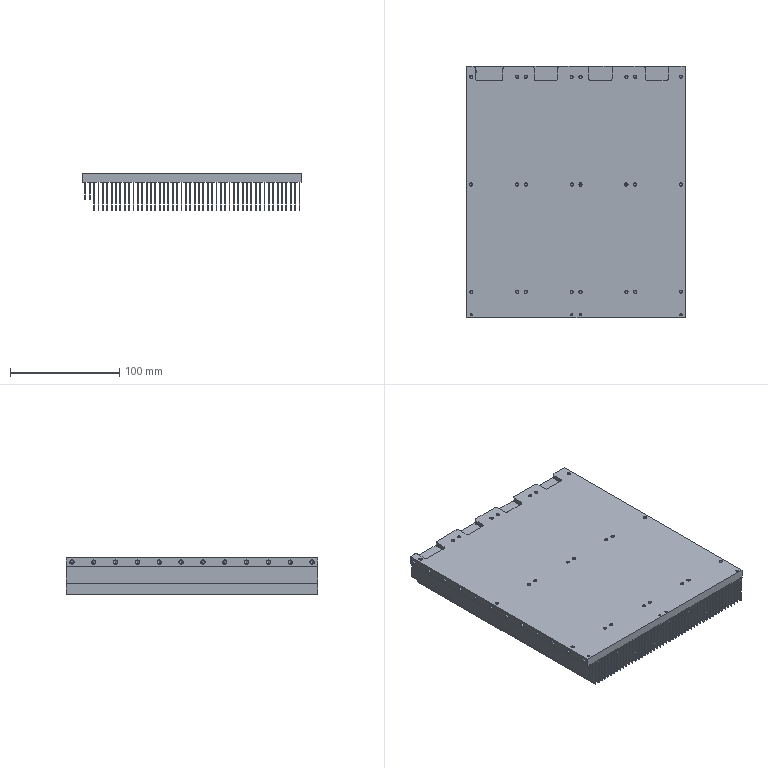Part | STEP file | SOLID | 1 solid | 377 faces | box 200 x 230 x 33.3 mm | volume 583013 mm3 | plane 222 | cone 92 | cylinder 63 | commonest cylinder face diameters 2.5 x25 3.3 x18 4 x16 1.6 x4